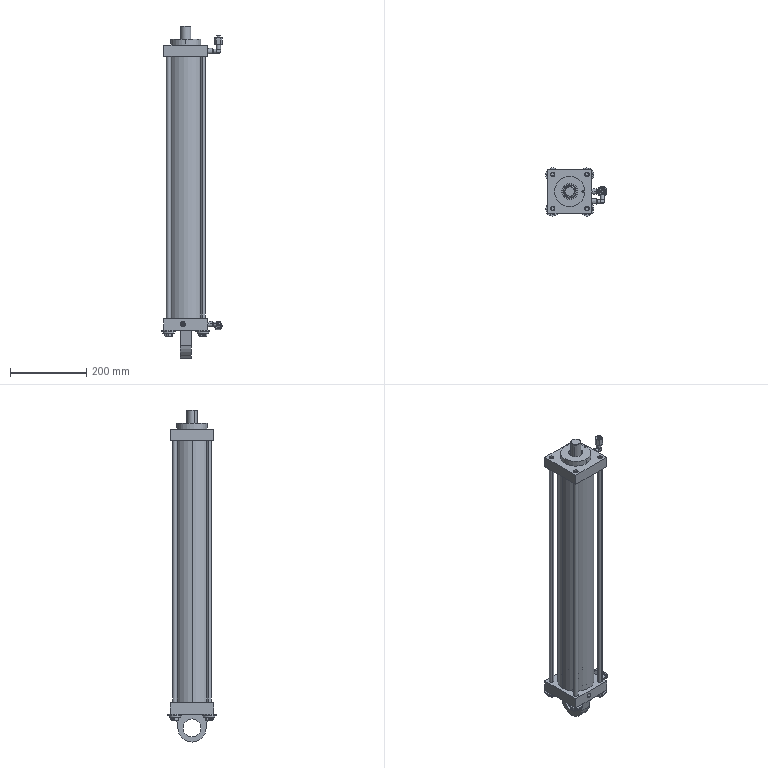Part | SolidWorks | features ReferencePattern 9, LocalCirPattern 1 | 19 solids | 585 faces | box 159.892 x 127 x 873 mm | volume 2737891 mm3 | cylinder 254 | plane 190 | cone 127 | torus 10 | sphere 2 | spline 2 | commonest cylinder face diameters 3.2 x32 6 x25 90 x18 12.5 x16 4 x12 20.2 x12